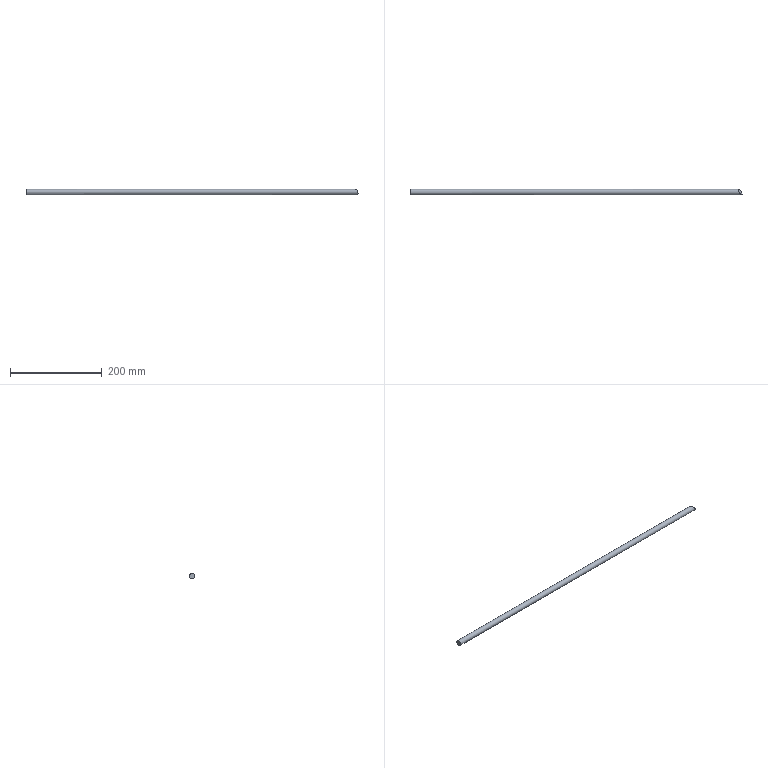Part | STEP file | solid 190 | 1 solid | 7 faces | box 724.85 x 12 x 12.001 mm | volume 81515 mm3 | spline 5 | cylinder 1 | plane 1 | commonest cylinder face diameters 12 x1